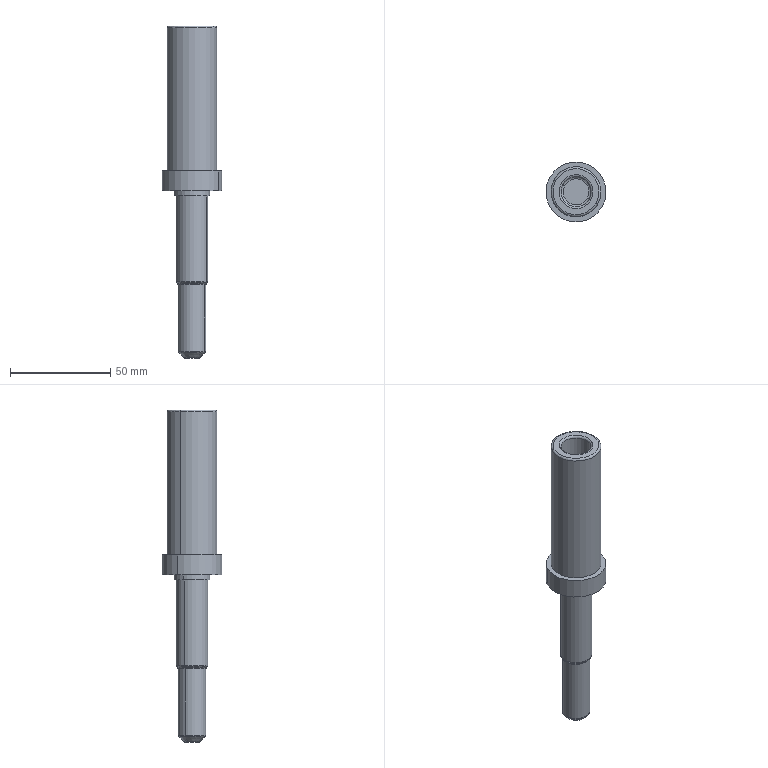Part | 1 solid | 36 faces | box 30 x 30 x 166 mm | volume 52321 mm3 | torus 14 | cylinder 12 | plane 6 | cone 4 | commonest cylinder face diameters 14 x2 15 x2 16 x2 18 x2 25 x2 30 x2